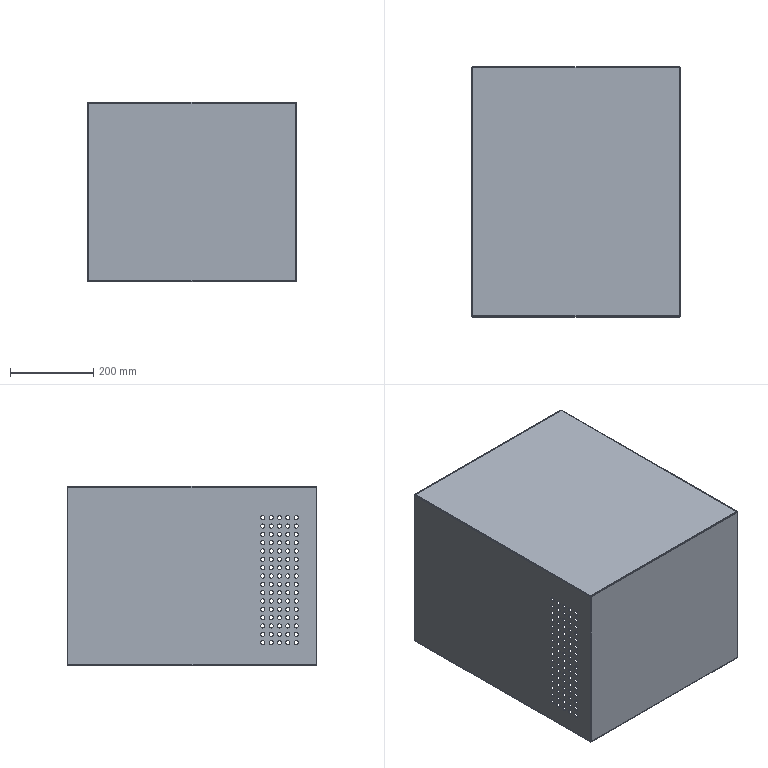Part | STEP file | X77-05401 | 1 solid | 744 faces | box 500 x 600 x 430 mm | volume 1547522 mm3 | cylinder 618 | plane 94 | spline 32 | commonest cylinder face diameters 10 x586 1.473 x16 3.873 x16